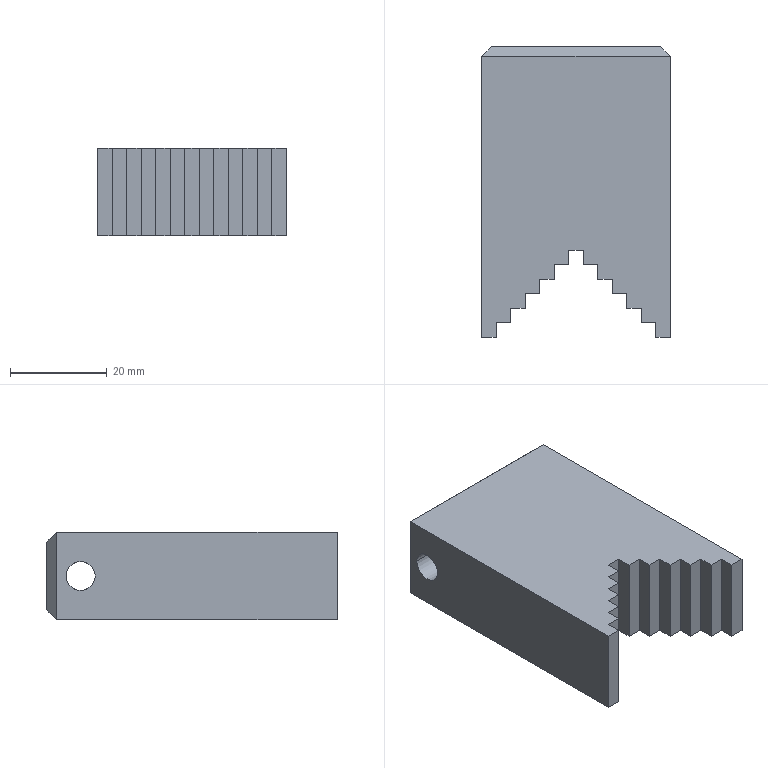Part | SolidWorks | features Chamfer 1, Extrusion 1, ICE 1, RevCut 1 | 1 solid | 42 faces | box 39 x 60 x 18 mm | volume 32904 mm3 | plane 34 | cylinder 6 | cone 2 | commonest cylinder face diameters 6 x4 12 x2
STEP:
#1=CARTESIAN_POINT('',(0.,0.2573,0.));
#2=VERTEX_POINT('',#1);
#3=CARTESIAN_POINT('',(0.,0.3937,0.2362));
#4=VERTEX_POINT('',#3);
#5=CARTESIAN_POINT('',(0.,0.2573,0.));
#6=DIRECTION('',(0.,0.5,0.866));
#7=VECTOR('',#6,39.37);
#8=LINE('',#5,#7);
#9=EDGE_CURVE('',#2,#4,#8,.T.);
#10=ORIENTED_EDGE('',*,*,#9,.F.);
#11=CARTESIAN_POINT('',(0.,0.3937,-0.2362));
#12=VERTEX_POINT('',#11);
#13=CARTESIAN_POINT('',(0.,0.2573,0.));
#14=DIRECTION('',(0.,0.5,-0.866));
#15=VECTOR('',#14,39.37);
#16=LINE('',#13,#15);
#17=EDGE_CURVE('',#2,#12,#16,.T.);
#18=ORIENTED_EDGE('',*,*,#17,.T.);
#19=CARTESIAN_POINT('',(0.,0.3937,0.));
#20=DIRECTION('',(0.,1.,0.));
#21=DIRECTION('',(0.,0.,1.));
#22=AXIS2_PLACEMENT_3D('',#19,#20,#21);
#23=CIRCLE('',#22,0.2362);
#24=EDGE_CURVE('',#12,#4,#23,.T.);
#25=ORIENTED_EDGE('',*,*,#24,.T.);
#26=EDGE_LOOP('',(#10,#18,#25));
#27=FACE_OUTER_BOUND('',#26,.T.);
#28=CARTESIAN_POINT('',(0.,39.627,0.));
#29=DIRECTION('',(0.,1.,0.));
#30=DIRECTION('',(0.,0.,1.));
#31=AXIS2_PLACEMENT_3D('',#28,#29,#30);
#32=CONICAL_SURFACE('',#31,68.191,1.047);
#33=ADVANCED_FACE('',(#27),#32,.F.);
#34=CARTESIAN_POINT('',(-0.2362,1.024,0.));
#35=VERTEX_POINT('',#34);
#36=CARTESIAN_POINT('',(-0.2362,0.7874,0.));
#37=VERTEX_POINT('',#36);
#38=CARTESIAN_POINT('',(-0.2362,1.024,0.));
#39=CARTESIAN_POINT('',(-0.2362,1.024,-0.007949));
#40=CARTESIAN_POINT('',(-0.2358,1.023,-0.01574));
#41=CARTESIAN_POINT('',(-0.2343,1.02,-0.03103));
#42=CARTESIAN_POINT('',(-0.2332,1.017,-0.0386));
#43=CARTESIAN_POINT('',(-0.2303,1.011,-0.05287));
#44=CARTESIAN_POINT('',(-0.2287,1.008,-0.05961));
#45=CARTESIAN_POINT('',(-0.225,0.9992,-0.07235));
#46=CARTESIAN_POINT('',(-0.223,0.9943,-0.07826));
#47=CARTESIAN_POINT('',(-0.2189,0.9836,-0.08896));
#48=CARTESIAN_POINT('',(-0.2168,0.9777,-0.09383));
#49=CARTESIAN_POINT('',(-0.2129,0.9649,-0.1024));
#50=CARTESIAN_POINT('',(-0.2111,0.9582,-0.106));
#51=CARTESIAN_POINT('',(-0.2081,0.9441,-0.1119));
#52=CARTESIAN_POINT('',(-0.2068,0.9365,-0.1142));
#53=CARTESIAN_POINT('',(-0.205,0.9212,-0.1173));
#54=CARTESIAN_POINT('',(-0.2046,0.9135,-0.1181));
#55=CARTESIAN_POINT('',(-0.2046,0.8978,-0.1181));
#56=CARTESIAN_POINT('',(-0.205,0.8898,-0.1173));
#57=CARTESIAN_POINT('',(-0.2068,0.8745,-0.1142));
#58=CARTESIAN_POINT('',(-0.208,0.867,-0.1119));
#59=CARTESIAN_POINT('',(-0.2112,0.8527,-0.1059));
#60=CARTESIAN_POINT('',(-0.213,0.846,-0.1023));
#61=CARTESIAN_POINT('',(-0.2169,0.8333,-0.09378));
#62=CARTESIAN_POINT('',(-0.2189,0.8274,-0.08888));
#63=CARTESIAN_POINT('',(-0.223,0.8166,-0.07817));
#64=CARTESIAN_POINT('',(-0.225,0.8118,-0.07231));
#65=CARTESIAN_POINT('',(-0.2287,0.8032,-0.05952));
#66=CARTESIAN_POINT('',(-0.2304,0.7996,-0.05274));
#67=CARTESIAN_POINT('',(-0.2332,0.7936,-0.03856));
#68=CARTESIAN_POINT('',(-0.2343,0.7913,-0.03106));
#69=CARTESIAN_POINT('',(-0.2358,0.7882,-0.01562));
#70=CARTESIAN_POINT('',(-0.2362,0.7874,-0.007842));
#71=CARTESIAN_POINT('',(-0.2362,0.7874,0.));
#72=B_SPLINE_CURVE_WITH_KNOTS('',3,(#38,#39,#40,#41,#42,#43,#44,#45,#46,#47,#48,#49,#50,#51,#52,#53,#54,#55,#56,#57,#58,#59,#60,#61,#62,#63,#64,#65,#66,#67,#68,#69,#70,#71),.UNSPECIFIED.,.F.,.F.,(4,2,2,2,2,2,2,2,2,2,2,2,2,2,2,2,4),(0.,0.0005964,0.001193,0.001789,0.002386,0.002982,0.003579,0.004175,0.004771,0.005368,0.005964,0.006561,0.007157,0.007754,0.00835,0.008947,0.009543),.UNSPECIFIED.);
#73=EDGE_CURVE('',#35,#37,#72,.T.);
#74=ORIENTED_EDGE('',*,*,#73,.T.);
#75=CARTESIAN_POINT('',(-0.2362,0.7874,0.));
#76=CARTESIAN_POINT('',(-0.2362,0.7874,0.007829));
#77=CARTESIAN_POINT('',(-0.2358,0.7882,0.0158));
#78=CARTESIAN_POINT('',(-0.2343,0.7913,0.0311));
#79=CARTESIAN_POINT('',(-0.2332,0.7936,0.03852));
#80=CARTESIAN_POINT('',(-0.2303,0.7996,0.05291));
#81=CARTESIAN_POINT('',(-0.2287,0.8033,0.05967));
#82=CARTESIAN_POINT('',(-0.225,0.8118,0.07232));
#83=CARTESIAN_POINT('',(-0.2229,0.8167,0.07827));
#84=CARTESIAN_POINT('',(-0.2189,0.8275,0.08899));
#85=CARTESIAN_POINT('',(-0.2169,0.8333,0.09379));
#86=CARTESIAN_POINT('',(-0.213,0.846,0.1023));
#87=CARTESIAN_POINT('',(-0.2111,0.8528,0.106));
#88=CARTESIAN_POINT('',(-0.2081,0.8669,0.1119));
#89=CARTESIAN_POINT('',(-0.2068,0.8743,0.1142));
#90=CARTESIAN_POINT('',(-0.205,0.8897,0.1173));
#91=CARTESIAN_POINT('',(-0.2046,0.8976,0.1181));
#92=CARTESIAN_POINT('',(-0.2046,0.9132,0.1181));
#93=CARTESIAN_POINT('',(-0.205,0.9211,0.1173));
#94=CARTESIAN_POINT('',(-0.2068,0.9365,0.1142));
#95=CARTESIAN_POINT('',(-0.208,0.9439,0.112));
#96=CARTESIAN_POINT('',(-0.2127,0.9653,0.103));
#97=CARTESIAN_POINT('',(-0.2169,0.9782,0.09436));
#98=CARTESIAN_POINT('',(-0.223,0.9943,0.07821));
#99=CARTESIAN_POINT('',(-0.225,0.9992,0.07237));
#100=CARTESIAN_POINT('',(-0.2286,1.008,0.05973));
#101=CARTESIAN_POINT('',(-0.2303,1.011,0.05285));
#102=CARTESIAN_POINT('',(-0.2332,1.017,0.03862));
#103=CARTESIAN_POINT('',(-0.2343,1.02,0.03124));
#104=CARTESIAN_POINT('',(-0.2358,1.023,0.01591));
#105=CARTESIAN_POINT('',(-0.2362,1.024,0.007935));
#106=CARTESIAN_POINT('',(-0.2362,1.024,0.));
#107=B_SPLINE_CURVE_WITH_KNOTS('',3,(#75,#76,#77,#78,#79,#80,#81,#82,#83,#84,#85,#86,#87,#88,#89,#90,#91,#92,#93,#94,#95,#96,#97,#98,#99,#100,#101,#102,#103,#104,#105,#106),.UNSPECIFIED.,.F.,.F.,(4,2,2,2,2,2,2,2,2,2,2,2,2,2,2,4),(0.009543,0.01014,0.01073,0.01133,0.01192,0.01252,0.01312,0.01371,0.01431,0.0149,0.0155,0.01669,0.01728,0.01788,0.01847,0.01907),.UNSPECIFIED.);
#108=EDGE_CURVE('',#37,#35,#107,.T.);
#109=ORIENTED_EDGE('',*,*,#108,.T.);
#110=EDGE_LOOP('',(#74,#109));
#111=FACE_BOUND('',#110,.T.);
#112=ORIENTED_EDGE('',*,*,#24,.F.);
#113=CARTESIAN_POINT('',(0.,1.181,-0.2362));
#114=VERTEX_POINT('',#113);
#115=CARTESIAN_POINT('',(0.,1.249,-0.2362));
#116=DIRECTION('',(0.,1.,0.));
#117=VECTOR('',#116,39.37);
#118=LINE('',#115,#117);
#119=EDGE_CURVE('',#12,#114,#118,.T.);
#120=ORIENTED_EDGE('',*,*,#119,.T.);
#121=CARTESIAN_POINT('',(0.,1.181,0.2362));
#122=VERTEX_POINT('',#121);
#123=CARTESIAN_POINT('',(0.,1.181,0.));
#124=DIRECTION('',(0.,1.,0.));
#125=DIRECTION('',(0.,0.,1.));
#126=AXIS2_PLACEMENT_3D('',#123,#124,#125);
#127=CIRCLE('',#126,0.2362);
#128=EDGE_CURVE('',#114,#122,#127,.T.);
#129=ORIENTED_EDGE('',*,*,#128,.T.);
#130=CARTESIAN_POINT('',(0.,1.249,0.2362));
#131=DIRECTION('',(0.,1.,0.));
#132=VECTOR('',#131,39.37);
#133=LINE('',#130,#132);
#134=EDGE_CURVE('',#4,#122,#133,.T.);
#135=ORIENTED_EDGE('',*,*,#134,.F.);
#136=EDGE_LOOP('',(#112,#120,#129,#135));
#137=FACE_OUTER_BOUND('',#136,.T.);
#138=CARTESIAN_POINT('',(0.,1.249,0.));
#139=DIRECTION('',(0.,1.,0.));
#140=DIRECTION('',(0.,0.,1.));
#141=AXIS2_PLACEMENT_3D('',#138,#139,#140);
#142=CYLINDRICAL_SURFACE('',#141,0.2362);
#143=ADVANCED_FACE('',(#111,#137),#142,.F.);
#144=CARTESIAN_POINT('',(0.2362,0.7874,0.));
#145=VERTEX_POINT('',#144);
#146=CARTESIAN_POINT('',(0.2362,1.024,0.));
#147=VERTEX_POINT('',#146);
#148=CARTESIAN_POINT('',(0.2362,0.7874,0.));
#149=CARTESIAN_POINT('',(0.2362,0.7874,-0.007829));
#150=CARTESIAN_POINT('',(0.2358,0.7882,-0.0158));
#151=CARTESIAN_POINT('',(0.2343,0.7913,-0.0311));
#152=CARTESIAN_POINT('',(0.2332,0.7936,-0.03852));
#153=CARTESIAN_POINT('',(0.2303,0.7996,-0.05291));
#154=CARTESIAN_POINT('',(0.2287,0.8033,-0.05967));
#155=CARTESIAN_POINT('',(0.225,0.8118,-0.07232));
#156=CARTESIAN_POINT('',(0.2229,0.8167,-0.07827));
#157=CARTESIAN_POINT('',(0.2189,0.8275,-0.08899));
#158=CARTESIAN_POINT('',(0.2169,0.8333,-0.09379));
#159=CARTESIAN_POINT('',(0.213,0.846,-0.1023));
#160=CARTESIAN_POINT('',(0.2111,0.8528,-0.106));
#161=CARTESIAN_POINT('',(0.2081,0.8669,-0.1119));
#162=CARTESIAN_POINT('',(0.2068,0.8743,-0.1142));
#163=CARTESIAN_POINT('',(0.205,0.8897,-0.1173));
#164=CARTESIAN_POINT('',(0.2046,0.8976,-0.1181));
#165=CARTESIAN_POINT('',(0.2046,0.9132,-0.1181));
#166=CARTESIAN_POINT('',(0.205,0.9211,-0.1173));
#167=CARTESIAN_POINT('',(0.2068,0.9365,-0.1142));
#168=CARTESIAN_POINT('',(0.208,0.9439,-0.112));
#169=CARTESIAN_POINT('',(0.2127,0.9653,-0.103));
#170=CARTESIAN_POINT('',(0.2169,0.9782,-0.09436));
#171=CARTESIAN_POINT('',(0.223,0.9943,-0.07821));
#172=CARTESIAN_POINT('',(0.225,0.9992,-0.07237));
#173=CARTESIAN_POINT('',(0.2286,1.008,-0.05973));
#174=CARTESIAN_POINT('',(0.2303,1.011,-0.05285));
#175=CARTESIAN_POINT('',(0.2332,1.017,-0.03862));
#176=CARTESIAN_POINT('',(0.2343,1.02,-0.03124));
#177=CARTESIAN_POINT('',(0.2358,1.023,-0.01591));
#178=CARTESIAN_POINT('',(0.2362,1.024,-0.007935));
#179=CARTESIAN_POINT('',(0.2362,1.024,0.));
#180=B_SPLINE_CURVE_WITH_KNOTS('',3,(#148,#149,#150,#151,#152,#153,#154,#155,#156,#157,#158,#159,#160,#161,#162,#163,#164,#165,#166,#167,#168,#169,#170,#171,#172,#173,#174,#175,#176,#177,#178,#179),.UNSPECIFIED.,.F.,.F.,(4,2,2,2,2,2,2,2,2,2,2,2,2,2,2,4),(0.009543,0.01014,0.01073,0.01133,0.01192,0.01252,0.01312,0.01371,0.01431,0.0149,0.0155,0.01669,0.01728,0.01788,0.01847,0.01907),.UNSPECIFIED.);
#181=EDGE_CURVE('',#145,#147,#180,.T.);
#182=ORIENTED_EDGE('',*,*,#181,.F.);
#183=CARTESIAN_POINT('',(0.7677,0.7874,0.));
#184=VERTEX_POINT('',#183);
#185=CARTESIAN_POINT('',(-0.7677,0.7874,0.));
#186=DIRECTION('',(1.,0.,0.));
#187=VECTOR('',#186,39.37);
#188=LINE('',#185,#187);
#189=EDGE_CURVE('',#145,#184,#188,.T.);
#190=ORIENTED_EDGE('',*,*,#189,.T.);
#191=CARTESIAN_POINT('',(0.7677,1.024,0.));
#192=VERTEX_POINT('',#191);
#193=CARTESIAN_POINT('',(0.7677,0.9055,0.));
#194=DIRECTION('',(1.,0.,0.));
#195=DIRECTION('',(0.,1.,0.));
#196=AXIS2_PLACEMENT_3D('',#193,#194,#195);
#197=CIRCLE('',#196,0.1181);
#198=EDGE_CURVE('',#184,#192,#197,.T.);
#199=ORIENTED_EDGE('',*,*,#198,.T.);
#200=CARTESIAN_POINT('',(-0.7677,1.024,0.));
#201=DIRECTION('',(1.,0.,0.));
#202=VECTOR('',#201,39.37);
#203=LINE('',#200,#202);
#204=EDGE_CURVE('',#147,#192,#203,.T.);
#205=ORIENTED_EDGE('',*,*,#204,.F.);
#206=EDGE_LOOP('',(#182,#190,#199,#205));
#207=FACE_OUTER_BOUND('',#206,.T.);
#208=CARTESIAN_POINT('',(-0.7677,0.9055,0.));
#209=DIRECTION('',(1.,0.,0.));
#210=DIRECTION('',(0.,1.,0.));
#211=AXIS2_PLACEMENT_3D('',#208,#209,#210);
#212=CYLINDRICAL_SURFACE('',#211,0.1181);
#213=ADVANCED_FACE('',(#207),#212,.F.);
#214=CARTESIAN_POINT('',(-0.7677,0.7874,0.));
#215=VERTEX_POINT('',#214);
#216=CARTESIAN_POINT('',(-0.7677,1.024,0.));
#217=VERTEX_POINT('',#216);
#218=CARTESIAN_POINT('',(-0.7677,0.9055,0.));
#219=DIRECTION('',(1.,0.,0.));
#220=DIRECTION('',(0.,1.,0.));
#221=AXIS2_PLACEMENT_3D('',#218,#219,#220);
#222=CIRCLE('',#221,0.1181);
#223=EDGE_CURVE('',#215,#217,#222,.T.);
#224=ORIENTED_EDGE('',*,*,#223,.F.);
#225=CARTESIAN_POINT('',(-0.7677,0.7874,0.));
#226=DIRECTION('',(1.,0.,0.));
#227=VECTOR('',#226,39.37);
#228=LINE('',#225,#227);
#229=EDGE_CURVE('',#215,#37,#228,.T.);
#230=ORIENTED_EDGE('',*,*,#229,.T.);
#231=ORIENTED_EDGE('',*,*,#73,.F.);
#232=CARTESIAN_POINT('',(-0.7677,1.024,0.));
#233=DIRECTION('',(1.,0.,0.));
#234=VECTOR('',#233,39.37);
#235=LINE('',#232,#234);
#236=EDGE_CURVE('',#217,#35,#235,.T.);
#237=ORIENTED_EDGE('',*,*,#236,.F.);
#238=EDGE_LOOP('',(#224,#230,#231,#237));
#239=FACE_OUTER_BOUND('',#238,.T.);
#240=CARTESIAN_POINT('',(-0.7677,0.9055,0.));
#241=DIRECTION('',(1.,0.,0.));
#242=DIRECTION('',(0.,1.,0.));
#243=AXIS2_PLACEMENT_3D('',#240,#241,#242);
#244=CYLINDRICAL_SURFACE('',#243,0.1181);
#245=ADVANCED_FACE('',(#239),#244,.F.);
#246=ORIENTED_EDGE('',*,*,#229,.F.);
#247=CARTESIAN_POINT('',(-0.7677,0.9055,0.));
#248=DIRECTION('',(1.,0.,0.));
#249=DIRECTION('',(0.,1.,0.));
#250=AXIS2_PLACEMENT_3D('',#247,#248,#249);
#251=CIRCLE('',#250,0.1181);
#252=EDGE_CURVE('',#217,#215,#251,.T.);
#253=ORIENTED_EDGE('',*,*,#252,.F.);
#254=ORIENTED_EDGE('',*,*,#236,.T.);
#255=ORIENTED_EDGE('',*,*,#108,.F.);
#256=EDGE_LOOP('',(#246,#253,#254,#255));
#257=FACE_OUTER_BOUND('',#256,.T.);
#258=CARTESIAN_POINT('',(-0.7677,0.9055,0.));
#259=DIRECTION('',(1.,0.,0.));
#260=DIRECTION('',(0.,1.,0.));
#261=AXIS2_PLACEMENT_3D('',#258,#259,#260);
#262=CYLINDRICAL_SURFACE('',#261,0.1181);
#263=ADVANCED_FACE('',(#257),#262,.F.);
#264=ORIENTED_EDGE('',*,*,#189,.F.);
#265=CARTESIAN_POINT('',(0.2362,1.024,0.));
#266=CARTESIAN_POINT('',(0.2362,1.024,0.007949));
#267=CARTESIAN_POINT('',(0.2358,1.023,0.01574));
#268=CARTESIAN_POINT('',(0.2343,1.02,0.03103));
#269=CARTESIAN_POINT('',(0.2332,1.017,0.0386));
#270=CARTESIAN_POINT('',(0.2303,1.011,0.05287));
#271=CARTESIAN_POINT('',(0.2287,1.008,0.05961));
#272=CARTESIAN_POINT('',(0.225,0.9992,0.07235));
#273=CARTESIAN_POINT('',(0.223,0.9943,0.07826));
#274=CARTESIAN_POINT('',(0.2189,0.9836,0.08896));
#275=CARTESIAN_POINT('',(0.2168,0.9777,0.09383));
#276=CARTESIAN_POINT('',(0.2129,0.9649,0.1024));
#277=CARTESIAN_POINT('',(0.2111,0.9582,0.106));
#278=CARTESIAN_POINT('',(0.2081,0.9441,0.1119));
#279=CARTESIAN_POINT('',(0.2068,0.9365,0.1142));
#280=CARTESIAN_POINT('',(0.205,0.9212,0.1173));
#281=CARTESIAN_POINT('',(0.2046,0.9135,0.1181));
#282=CARTESIAN_POINT('',(0.2046,0.8978,0.1181));
#283=CARTESIAN_POINT('',(0.205,0.8898,0.1173));
#284=CARTESIAN_POINT('',(0.2068,0.8745,0.1142));
#285=CARTESIAN_POINT('',(0.208,0.867,0.1119));
#286=CARTESIAN_POINT('',(0.2112,0.8527,0.1059));
#287=CARTESIAN_POINT('',(0.213,0.846,0.1023));
#288=CARTESIAN_POINT('',(0.2169,0.8333,0.09378));
#289=CARTESIAN_POINT('',(0.2189,0.8274,0.08888));
#290=CARTESIAN_POINT('',(0.223,0.8166,0.07817));
#291=CARTESIAN_POINT('',(0.225,0.8118,0.07231));
#292=CARTESIAN_POINT('',(0.2287,0.8032,0.05952));
#293=CARTESIAN_POINT('',(0.2304,0.7996,0.05274));
#294=CARTESIAN_POINT('',(0.2332,0.7936,0.03856));
#295=CARTESIAN_POINT('',(0.2343,0.7913,0.03106));
#296=CARTESIAN_POINT('',(0.2358,0.7882,0.01562));
#297=CARTESIAN_POINT('',(0.2362,0.7874,0.007842));
#298=CARTESIAN_POINT('',(0.2362,0.7874,0.));
#299=B_SPLINE_CURVE_WITH_KNOTS('',3,(#265,#266,#267,#268,#269,#270,#271,#272,#273,#274,#275,#276,#277,#278,#279,#280,#281,#282,#283,#284,#285,#286,#287,#288,#289,#290,#291,#292,#293,#294,#295,#296,#297,#298),.UNSPECIFIED.,.F.,.F.,(4,2,2,2,2,2,2,2,2,2,2,2,2,2,2,2,4),(0.,0.0005964,0.001193,0.001789,0.002386,0.002982,0.003579,0.004175,0.004771,0.005368,0.005964,0.006561,0.007157,0.007754,0.00835,0.008947,0.009543),.UNSPECIFIED.);
#300=EDGE_CURVE('',#147,#145,#299,.T.);
#301=ORIENTED_EDGE('',*,*,#300,.F.);
#302=ORIENTED_EDGE('',*,*,#204,.T.);
#303=CARTESIAN_POINT('',(0.7677,0.9055,0.));
#304=DIRECTION('',(1.,0.,0.));
#305=DIRECTION('',(0.,1.,0.));
#306=AXIS2_PLACEMENT_3D('',#303,#304,#305);
#307=CIRCLE('',#306,0.1181);
#308=EDGE_CURVE('',#192,#184,#307,.T.);
#309=ORIENTED_EDGE('',*,*,#308,.T.);
#310=EDGE_LOOP('',(#264,#301,#302,#309));
#311=FACE_OUTER_BOUND('',#310,.T.);
#312=CARTESIAN_POINT('',(-0.7677,0.9055,0.));
#313=DIRECTION('',(1.,0.,0.));
#314=DIRECTION('',(0.,1.,0.));
#315=AXIS2_PLACEMENT_3D('',#312,#313,#314);
#316=CYLINDRICAL_SURFACE('',#315,0.1181);
#317=ADVANCED_FACE('',(#311),#316,.F.);
#318=CARTESIAN_POINT('',(0.6496,-1.181,-0.3543));
#319=VERTEX_POINT('',#318);
#320=CARTESIAN_POINT('',(0.7677,-1.181,-0.3543));
#321=VERTEX_POINT('',#320);
#322=CARTESIAN_POINT('',(0.6496,-1.181,-0.3543));
#323=DIRECTION('',(1.,0.,0.));
#324=VECTOR('',#323,39.37);
#325=LINE('',#322,#324);
#326=EDGE_CURVE('',#319,#321,#325,.T.);
#327=ORIENTED_EDGE('',*,*,#326,.T.);
#328=CARTESIAN_POINT('',(0.7677,-1.181,0.3543));
#329=VERTEX_POINT('',#328);
#330=CARTESIAN_POINT('',(0.7677,-1.181,0.3543));
#331=DIRECTION('',(0.,0.,-1.));
#332=VECTOR('',#331,39.37);
#333=LINE('',#330,#332);
#334=EDGE_CURVE('',#329,#321,#333,.T.);
#335=ORIENTED_EDGE('',*,*,#334,.F.);
#336=CARTESIAN_POINT('',(0.6496,-1.181,0.3543));
#337=VERTEX_POINT('',#336);
#338=CARTESIAN_POINT('',(0.6496,-1.181,0.3543));
#339=DIRECTION('',(1.,0.,0.));
#340=VECTOR('',#339,39.37);
#341=LINE('',#338,#340);
#342=EDGE_CURVE('',#337,#329,#341,.T.);
#343=ORIENTED_EDGE('',*,*,#342,.F.);
#344=CARTESIAN_POINT('',(0.6496,-1.181,0.3543));
#345=DIRECTION('',(0.,0.,-1.));
#346=VECTOR('',#345,39.37);
#347=LINE('',#344,#346);
#348=EDGE_CURVE('',#337,#319,#347,.T.);
#349=ORIENTED_EDGE('',*,*,#348,.T.);
#350=EDGE_LOOP('',(#327,#335,#343,#349));
#351=FACE_OUTER_BOUND('',#350,.T.);
#352=CARTESIAN_POINT('',(0.6496,-1.181,0.3543));
#353=DIRECTION('',(0.,1.,0.));
#354=DIRECTION('',(0.,0.,1.));
#355=AXIS2_PLACEMENT_3D('',#352,#353,#354);
#356=PLANE('',#355);
#357=ADVANCED_FACE('',(#351),#356,.F.);
#358=ORIENTED_EDGE('',*,*,#308,.F.);
#359=ORIENTED_EDGE('',*,*,#198,.F.);
#360=EDGE_LOOP('',(#358,#359));
#361=FACE_BOUND('',#360,.T.);
#362=CARTESIAN_POINT('',(0.7677,1.102,-0.3543));
#363=VERTEX_POINT('',#362);
#364=CARTESIAN_POINT('',(0.7677,1.181,-0.3543));
#365=DIRECTION('',(0.,1.,0.));
#366=VECTOR('',#365,39.37);
#367=LINE('',#364,#366);
#368=EDGE_CURVE('',#321,#363,#367,.T.);
#369=ORIENTED_EDGE('',*,*,#368,.T.);
#370=CARTESIAN_POINT('',(0.7677,1.102,0.3543));
#371=VERTEX_POINT('',#370);
#372=CARTESIAN_POINT('',(0.7677,1.102,0.3543));
#373=DIRECTION('',(0.,0.,1.));
#374=VECTOR('',#373,39.37);
#375=LINE('',#372,#374);
#376=EDGE_CURVE('',#363,#371,#375,.T.);
#377=ORIENTED_EDGE('',*,*,#376,.T.);
#378=CARTESIAN_POINT('',(0.7677,1.181,0.3543));
#379=DIRECTION('',(0.,1.,0.));
#380=VECTOR('',#379,39.37);
#381=LINE('',#378,#380);
#382=EDGE_CURVE('',#329,#371,#381,.T.);
#383=ORIENTED_EDGE('',*,*,#382,.F.);
#384=ORIENTED_EDGE('',*,*,#334,.T.);
#385=EDGE_LOOP('',(#369,#377,#383,#384));
#386=FACE_OUTER_BOUND('',#385,.T.);
#387=CARTESIAN_POINT('',(0.7677,1.181,0.3543));
#388=DIRECTION('',(-1.,0.,0.));
#389=DIRECTION('',(0.,-1.,0.));
#390=AXIS2_PLACEMENT_3D('',#387,#388,#389);
#391=PLANE('',#390);
#392=ADVANCED_FACE('',(#361,#386),#391,.F.);
#393=CARTESIAN_POINT('',(0.,1.181,0.));
#394=DIRECTION('',(0.,1.,0.));
#395=DIRECTION('',(0.,0.,1.));
#396=AXIS2_PLACEMENT_3D('',#393,#394,#395);
#397=CIRCLE('',#396,0.2362);
#398=EDGE_CURVE('',#122,#114,#397,.T.);
#399=ORIENTED_EDGE('',*,*,#398,.F.);
#400=ORIENTED_EDGE('',*,*,#128,.F.);
#401=EDGE_LOOP('',(#399,#400));
#402=FACE_BOUND('',#401,.T.);
#403=CARTESIAN_POINT('',(-0.689,1.181,0.2756));
#404=VERTEX_POINT('',#403);
#405=CARTESIAN_POINT('',(0.689,1.181,0.2756));
#406=VERTEX_POINT('',#405);
#407=CARTESIAN_POINT('',(-0.7677,1.181,0.2756));
#408=DIRECTION('',(1.,0.,0.));
#409=VECTOR('',#408,39.37);
#410=LINE('',#407,#409);
#411=EDGE_CURVE('',#404,#406,#410,.T.);
#412=ORIENTED_EDGE('',*,*,#411,.T.);
#413=CARTESIAN_POINT('',(0.689,1.181,-0.2756));
#414=VERTEX_POINT('',#413);
#415=CARTESIAN_POINT('',(0.689,1.181,0.3543));
#416=DIRECTION('',(0.,0.,-1.));
#417=VECTOR('',#416,39.37);
#418=LINE('',#415,#417);
#419=EDGE_CURVE('',#406,#414,#418,.T.);
#420=ORIENTED_EDGE('',*,*,#419,.T.);
#421=CARTESIAN_POINT('',(-0.689,1.181,-0.2756));
#422=VERTEX_POINT('',#421);
#423=CARTESIAN_POINT('',(-0.7677,1.181,-0.2756));
#424=DIRECTION('',(-1.,0.,0.));
#425=VECTOR('',#424,39.37);
#426=LINE('',#423,#425);
#427=EDGE_CURVE('',#414,#422,#426,.T.);
#428=ORIENTED_EDGE('',*,*,#427,.T.);
#429=CARTESIAN_POINT('',(-0.689,1.181,0.3543));
#430=DIRECTION('',(0.,0.,1.));
#431=VECTOR('',#430,39.37);
#432=LINE('',#429,#431);
#433=EDGE_CURVE('',#422,#404,#432,.T.);
#434=ORIENTED_EDGE('',*,*,#433,.T.);
#435=EDGE_LOOP('',(#412,#420,#428,#434));
#436=FACE_OUTER_BOUND('',#435,.T.);
#437=CARTESIAN_POINT('',(-0.7677,1.181,0.3543));
#438=DIRECTION('',(0.,-1.,0.));
#439=DIRECTION('',(0.,0.,-1.));
#440=AXIS2_PLACEMENT_3D('',#437,#438,#439);
#441=PLANE('',#440);
#442=ADVANCED_FACE('',(#402,#436),#441,.F.);
#443=ORIENTED_EDGE('',*,*,#252,.T.);
#444=ORIENTED_EDGE('',*,*,#223,.T.);
#445=EDGE_LOOP('',(#443,#444));
#446=FACE_BOUND('',#445,.T.);
#447=CARTESIAN_POINT('',(-0.7677,1.102,0.3543));
#448=VERTEX_POINT('',#447);
#449=CARTESIAN_POINT('',(-0.7677,-1.181,0.3543));
#450=VERTEX_POINT('',#449);
#451=CARTESIAN_POINT('',(-0.7677,1.181,0.3543));
#452=DIRECTION('',(0.,-1.,0.));
#453=VECTOR('',#452,39.37);
#454=LINE('',#451,#453);
#455=EDGE_CURVE('',#448,#450,#454,.T.);
#456=ORIENTED_EDGE('',*,*,#455,.F.);
#457=CARTESIAN_POINT('',(-0.7677,1.102,-0.3543));
#458=VERTEX_POINT('',#457);
#459=CARTESIAN_POINT('',(-0.7677,1.102,0.3543));
#460=DIRECTION('',(0.,0.,-1.));
#461=VECTOR('',#460,39.37);
#462=LINE('',#459,#461);
#463=EDGE_CURVE('',#448,#458,#462,.T.);
#464=ORIENTED_EDGE('',*,*,#463,.T.);
#465=CARTESIAN_POINT('',(-0.7677,-1.181,-0.3543));
#466=VERTEX_POINT('',#465);
#467=CARTESIAN_POINT('',(-0.7677,1.181,-0.3543));
#468=DIRECTION('',(0.,-1.,0.));
#469=VECTOR('',#468,39.37);
#470=LINE('',#467,#469);
#471=EDGE_CURVE('',#458,#466,#470,.T.);
#472=ORIENTED_EDGE('',*,*,#471,.T.);
#473=CARTESIAN_POINT('',(-0.7677,-1.181,0.3543));
#474=DIRECTION('',(0.,0.,-1.));
#475=VECTOR('',#474,39.37);
#476=LINE('',#473,#475);
#477=EDGE_CURVE('',#450,#466,#476,.T.);
#478=ORIENTED_EDGE('',*,*,#477,.F.);
#479=EDGE_LOOP('',(#456,#464,#472,#478));
#480=FACE_OUTER_BOUND('',#479,.T.);
#481=CARTESIAN_POINT('',(-0.7677,1.181,0.3543));
#482=DIRECTION('',(1.,0.,0.));
#483=DIRECTION('',(0.,1.,0.));
#484=AXIS2_PLACEMENT_3D('',#481,#482,#483);
#485=PLANE('',#484);
#486=ADVANCED_FACE('',(#446,#480),#485,.F.);
#487=CARTESIAN_POINT('',(-0.6496,-1.181,-0.3543));
#488=VERTEX_POINT('',#487);
#489=CARTESIAN_POINT('',(-0.7677,-1.181,-0.3543));
#490=DIRECTION('',(1.,0.,0.));
#491=VECTOR('',#490,39.37);
#492=LINE('',#489,#491);
#493=EDGE_CURVE('',#466,#488,#492,.T.);
#494=ORIENTED_EDGE('',*,*,#493,.T.);
#495=CARTESIAN_POINT('',(-0.6496,-1.181,0.3543));
#496=VERTEX_POINT('',#495);
#497=CARTESIAN_POINT('',(-0.6496,-1.181,0.3543));
#498=DIRECTION('',(0.,0.,-1.));
#499=VECTOR('',#498,39.37);
#500=LINE('',#497,#499);
#501=EDGE_CURVE('',#496,#488,#500,.T.);
#502=ORIENTED_EDGE('',*,*,#501,.F.);
#503=CARTESIAN_POINT('',(-0.7677,-1.181,0.3543));
#504=DIRECTION('',(1.,0.,0.));
#505=VECTOR('',#504,39.37);
#506=LINE('',#503,#505);
#507=EDGE_CURVE('',#450,#496,#506,.T.);
#508=ORIENTED_EDGE('',*,*,#507,.F.);
#509=ORIENTED_EDGE('',*,*,#477,.T.);
#510=EDGE_LOOP('',(#494,#502,#508,#509));
#511=FACE_OUTER_BOUND('',#510,.T.);
#512=CARTESIAN_POINT('',(-0.7677,-1.181,0.3543));
#513=DIRECTION('',(0.,1.,0.));
#514=DIRECTION('',(0.,0.,1.));
#515=AXIS2_PLACEMENT_3D('',#512,#513,#514);
#516=PLANE('',#515);
#517=ADVANCED_FACE('',(#511),#516,.F.);
#518=CARTESIAN_POINT('',(-0.6496,-1.063,-0.3543));
#519=VERTEX_POINT('',#518);
#520=CARTESIAN_POINT('',(-0.6496,-1.181,-0.3543));
#521=DIRECTION('',(0.,1.,0.));
#522=VECTOR('',#521,39.37);
#523=LINE('',#520,#522);
#524=EDGE_CURVE('',#488,#519,#523,.T.);
#525=ORIENTED_EDGE('',*,*,#524,.T.);
#526=CARTESIAN_POINT('',(-0.6496,-1.063,0.3543));
#527=VERTEX_POINT('',#526);
#528=CARTESIAN_POINT('',(-0.6496,-1.063,0.3543));
#529=DIRECTION('',(0.,0.,-1.));
#530=VECTOR('',#529,39.37);
#531=LINE('',#528,#530);
#532=EDGE_CURVE('',#527,#519,#531,.T.);
#533=ORIENTED_EDGE('',*,*,#532,.F.);
#534=CARTESIAN_POINT('',(-0.6496,-1.181,0.3543));
#535=DIRECTION('',(0.,1.,0.));
#536=VECTOR('',#535,39.37);
#537=LINE('',#534,#536);
#538=EDGE_CURVE('',#496,#527,#537,.T.);
#539=ORIENTED_EDGE('',*,*,#538,.F.);
#540=ORIENTED_EDGE('',*,*,#501,.T.);
#541=EDGE_LOOP('',(#525,#533,#539,#540));
#542=FACE_OUTER_BOUND('',#541,.T.);
#543=CARTESIAN_POINT('',(-0.6496,-1.181,0.3543));
#544=DIRECTION('',(-1.,0.,0.));
#545=DIRECTION('',(0.,0.,1.));
#546=AXIS2_PLACEMENT_3D('',#543,#544,#545);
#547=PLANE('',#546);
#548=ADVANCED_FACE('',(#542),#547,.F.);
#549=CARTESIAN_POINT('',(-0.5315,-1.063,-0.3543));
#550=VERTEX_POINT('',#549);
#551=CARTESIAN_POINT('',(-0.6496,-1.063,-0.3543));
#552=DIRECTION('',(1.,0.,0.));
#553=VECTOR('',#552,39.37);
#554=LINE('',#551,#553);
#555=EDGE_CURVE('',#519,#550,#554,.T.);
#556=ORIENTED_EDGE('',*,*,#555,.T.);
#557=CARTESIAN_POINT('',(-0.5315,-1.063,0.3543));
#558=VERTEX_POINT('',#557);
#559=CARTESIAN_POINT('',(-0.5315,-1.063,0.3543));
#560=DIRECTION('',(0.,0.,-1.));
#561=VECTOR('',#560,39.37);
#562=LINE('',#559,#561);
#563=EDGE_CURVE('',#558,#550,#562,.T.);
#564=ORIENTED_EDGE('',*,*,#563,.F.);
#565=CARTESIAN_POINT('',(-0.6496,-1.063,0.3543));
#566=DIRECTION('',(1.,0.,0.));
#567=VECTOR('',#566,39.37);
#568=LINE('',#565,#567);
#569=EDGE_CURVE('',#527,#558,#568,.T.);
#570=ORIENTED_EDGE('',*,*,#569,.F.);
#571=ORIENTED_EDGE('',*,*,#532,.T.);
#572=EDGE_LOOP('',(#556,#564,#570,#571));
#573=FACE_OUTER_BOUND('',#572,.T.);
#574=CARTESIAN_POINT('',(-0.6496,-1.063,0.3543));
#575=DIRECTION('',(0.,1.,0.));
#576=DIRECTION('',(0.,0.,1.));
#577=AXIS2_PLACEMENT_3D('',#574,#575,#576);
#578=PLANE('',#577);
#579=ADVANCED_FACE('',(#573),#578,.F.);
#580=CARTESIAN_POINT('',(-0.5315,-0.9449,-0.3543));
#581=VERTEX_POINT('',#580);
#582=CARTESIAN_POINT('',(-0.5315,-1.063,-0.3543));
#583=DIRECTION('',(0.,1.,0.));
#584=VECTOR('',#583,39.37);
#585=LINE('',#582,#584);
#586=EDGE_CURVE('',#550,#581,#585,.T.);
#587=ORIENTED_EDGE('',*,*,#586,.T.);
#588=CARTESIAN_POINT('',(-0.5315,-0.9449,0.3543));
#589=VERTEX_POINT('',#588);
#590=CARTESIAN_POINT('',(-0.5315,-0.9449,0.3543));
#591=DIRECTION('',(0.,0.,-1.));
#592=VECTOR('',#591,39.37);
#593=LINE('',#590,#592);
#594=EDGE_CURVE('',#589,#581,#593,.T.);
#595=ORIENTED_EDGE('',*,*,#594,.F.);
#596=CARTESIAN_POINT('',(-0.5315,-1.063,0.3543));
#597=DIRECTION('',(0.,1.,0.));
#598=VECTOR('',#597,39.37);
#599=LINE('',#596,#598);
#600=EDGE_CURVE('',#558,#589,#599,.T.);
#601=ORIENTED_EDGE('',*,*,#600,.F.);
#602=ORIENTED_EDGE('',*,*,#563,.T.);
#603=EDGE_LOOP('',(#587,#595,#601,#602));
#604=FACE_OUTER_BOUND('',#603,.T.);
#605=CARTESIAN_POINT('',(-0.5315,-1.063,0.3543));
#606=DIRECTION('',(-1.,0.,0.));
#607=DIRECTION('',(0.,0.,1.));
#608=AXIS2_PLACEMENT_3D('',#605,#606,#607);
#609=PLANE('',#608);
#610=ADVANCED_FACE('',(#604),#609,.F.);
#611=CARTESIAN_POINT('',(-0.4134,-0.9449,-0.3543));
#612=VERTEX_POINT('',#611);
#613=CARTESIAN_POINT('',(-0.5315,-0.9449,-0.3543));
#614=DIRECTION('',(1.,0.,0.));
#615=VECTOR('',#614,39.37);
#616=LINE('',#613,#615);
#617=EDGE_CURVE('',#581,#612,#616,.T.);
#618=ORIENTED_EDGE('',*,*,#617,.T.);
#619=CARTESIAN_POINT('',(-0.4134,-0.9449,0.3543));
#620=VERTEX_POINT('',#619);
#621=CARTESIAN_POINT('',(-0.4134,-0.9449,0.3543));
#622=DIRECTION('',(0.,0.,-1.));
#623=VECTOR('',#622,39.37);
#624=LINE('',#621,#623);
#625=EDGE_CURVE('',#620,#612,#624,.T.);
#626=ORIENTED_EDGE('',*,*,#625,.F.);
#627=CARTESIAN_POINT('',(-0.5315,-0.9449,0.3543));
#628=DIRECTION('',(1.,0.,0.));
#629=VECTOR('',#628,39.37);
#630=LINE('',#627,#629);
#631=EDGE_CURVE('',#589,#620,#630,.T.);
#632=ORIENTED_EDGE('',*,*,#631,.F.);
#633=ORIENTED_EDGE('',*,*,#594,.T.);
#634=EDGE_LOOP('',(#618,#626,#632,#633));
#635=FACE_OUTER_BOUND('',#634,.T.);
#636=CARTESIAN_POINT('',(-0.5315,-0.9449,0.3543));
#637=DIRECTION('',(0.,1.,0.));
#638=DIRECTION('',(0.,0.,1.));
#639=AXIS2_PLACEMENT_3D('',#636,#637,#638);
#640=PLANE('',#639);
#641=ADVANCED_FACE('',(#635),#640,.F.);
#642=CARTESIAN_POINT('',(-0.4134,-0.8268,-0.3543));
#643=VERTEX_POINT('',#642);
#644=CARTESIAN_POINT('',(-0.4134,-0.9449,-0.3543));
#645=DIRECTION('',(0.,1.,0.));
#646=VECTOR('',#645,39.37);
#647=LINE('',#644,#646);
#648=EDGE_CURVE('',#612,#643,#647,.T.);
#649=ORIENTED_EDGE('',*,*,#648,.T.);
#650=CARTESIAN_POINT('',(-0.4134,-0.8268,0.3543));
#651=VERTEX_POINT('',#650);
#652=CARTESIAN_POINT('',(-0.4134,-0.8268,0.3543));
#653=DIRECTION('',(0.,0.,-1.));
#654=VECTOR('',#653,39.37);
#655=LINE('',#652,#654);
#656=EDGE_CURVE('',#651,#643,#655,.T.);
#657=ORIENTED_EDGE('',*,*,#656,.F.);
#658=CARTESIAN_POINT('',(-0.4134,-0.9449,0.3543));
#659=DIRECTION('',(0.,1.,0.));
#660=VECTOR('',#659,39.37);
#661=LINE('',#658,#660);
#662=EDGE_CURVE('',#620,#651,#661,.T.);
#663=ORIENTED_EDGE('',*,*,#662,.F.);
#664=ORIENTED_EDGE('',*,*,#625,.T.);
#665=EDGE_LOOP('',(#649,#657,#663,#664));
#666=FACE_OUTER_BOUND('',#665,.T.);
#667=CARTESIAN_POINT('',(-0.4134,-0.9449,0.3543));
#668=DIRECTION('',(-1.,0.,0.));
#669=DIRECTION('',(0.,0.,1.));
#670=AXIS2_PLACEMENT_3D('',#667,#668,#669);
#671=PLANE('',#670);
#672=ADVANCED_FACE('',(#666),#671,.F.);
#673=CARTESIAN_POINT('',(-0.2953,-0.8268,-0.3543));
#674=VERTEX_POINT('',#673);
#675=CARTESIAN_POINT('',(-0.4134,-0.8268,-0.3543));
#676=DIRECTION('',(1.,0.,0.));
#677=VECTOR('',#676,39.37);
#678=LINE('',#675,#677);
#679=EDGE_CURVE('',#643,#674,#678,.T.);
#680=ORIENTED_EDGE('',*,*,#679,.T.);
#681=CARTESIAN_POINT('',(-0.2953,-0.8268,0.3543));
#682=VERTEX_POINT('',#681);
#683=CARTESIAN_POINT('',(-0.2953,-0.8268,0.3543));
#684=DIRECTION('',(0.,0.,-1.));
#685=VECTOR('',#684,39.37);
#686=LINE('',#683,#685);
#687=EDGE_CURVE('',#682,#674,#686,.T.);
#688=ORIENTED_EDGE('',*,*,#687,.F.);
#689=CARTESIAN_POINT('',(-0.4134,-0.8268,0.3543));
#690=DIRECTION('',(1.,0.,0.));
#691=VECTOR('',#690,39.37);
#692=LINE('',#689,#691);
#693=EDGE_CURVE('',#651,#682,#692,.T.);
#694=ORIENTED_EDGE('',*,*,#693,.F.);
#695=ORIENTED_EDGE('',*,*,#656,.T.);
#696=EDGE_LOOP('',(#680,#688,#694,#695));
#697=FACE_OUTER_BOUND('',#696,.T.);
#698=CARTESIAN_POINT('',(-0.4134,-0.8268,0.3543));
#699=DIRECTION('',(0.,1.,0.));
#700=DIRECTION('',(0.,0.,1.));
#701=AXIS2_PLACEMENT_3D('',#698,#699,#700);
#702=PLANE('',#701);
#703=ADVANCED_FACE('',(#697),#702,.F.);
#704=CARTESIAN_POINT('',(-0.2953,-0.7087,-0.3543));
#705=VERTEX_POINT('',#704);
#706=CARTESIAN_POINT('',(-0.2953,-0.8268,-0.3543));
#707=DIRECTION('',(0.,1.,0.));
#708=VECTOR('',#707,39.37);
#709=LINE('',#706,#708);
#710=EDGE_CURVE('',#674,#705,#709,.T.);
#711=ORIENTED_EDGE('',*,*,#710,.T.);
#712=CARTESIAN_POINT('',(-0.2953,-0.7087,0.3543));
#713=VERTEX_POINT('',#712);
#714=CARTESIAN_POINT('',(-0.2953,-0.7087,0.3543));
#715=DIRECTION('',(0.,0.,-1.));
#716=VECTOR('',#715,39.37);
#717=LINE('',#714,#716);
#718=EDGE_CURVE('',#713,#705,#717,.T.);
#719=ORIENTED_EDGE('',*,*,#718,.F.);
#720=CARTESIAN_POINT('',(-0.2953,-0.8268,0.3543));
#721=DIRECTION('',(0.,1.,0.));
#722=VECTOR('',#721,39.37);
#723=LINE('',#720,#722);
#724=EDGE_CURVE('',#682,#713,#723,.T.);
#725=ORIENTED_EDGE('',*,*,#724,.F.);
#726=ORIENTED_EDGE('',*,*,#687,.T.);
#727=EDGE_LOOP('',(#711,#719,#725,#726));
#728=FACE_OUTER_BOUND('',#727,.T.);
#729=CARTESIAN_POINT('',(-0.2953,-0.8268,0.3543));
#730=DIRECTION('',(-1.,0.,0.));
#731=DIRECTION('',(0.,0.,1.));
#732=AXIS2_PLACEMENT_3D('',#729,#730,#731);
#733=PLANE('',#732);
#734=ADVANCED_FACE('',(#728),#733,.F.);
#735=CARTESIAN_POINT('',(-0.1772,-0.7087,-0.3543));
#736=VERTEX_POINT('',#735);
#737=CARTESIAN_POINT('',(-0.2953,-0.7087,-0.3543));
#738=DIRECTION('',(1.,0.,0.));
#739=VECTOR('',#738,39.37);
#740=LINE('',#737,#739);
#741=EDGE_CURVE('',#705,#736,#740,.T.);
#742=ORIENTED_EDGE('',*,*,#741,.T.);
#743=CARTESIAN_POINT('',(-0.1772,-0.7087,0.3543));
#744=VERTEX_POINT('',#743);
#745=CARTESIAN_POINT('',(-0.1772,-0.7087,0.3543));
#746=DIRECTION('',(0.,0.,-1.));
#747=VECTOR('',#746,39.37);
#748=LINE('',#745,#747);
#749=EDGE_CURVE('',#744,#736,#748,.T.);
#750=ORIENTED_EDGE('',*,*,#749,.F.);
#751=CARTESIAN_POINT('',(-0.2953,-0.7087,0.3543));
#752=DIRECTION('',(1.,0.,0.));
#753=VECTOR('',#752,39.37);
#754=LINE('',#751,#753);
#755=EDGE_CURVE('',#713,#744,#754,.T.);
#756=ORIENTED_EDGE('',*,*,#755,.F.);
#757=ORIENTED_EDGE('',*,*,#718,.T.);
#758=EDGE_LOOP('',(#742,#750,#756,#757));
#759=FACE_OUTER_BOUND('',#758,.T.);
#760=CARTESIAN_POINT('',(-0.2953,-0.7087,0.3543));
#761=DIRECTION('',(0.,1.,0.));
#762=DIRECTION('',(0.,0.,1.));
#763=AXIS2_PLACEMENT_3D('',#760,#761,#762);
#764=PLANE('',#763);
#765=ADVANCED_FACE('',(#759),#764,.F.);
#766=CARTESIAN_POINT('',(-0.1772,-0.5906,-0.3543));
#767=VERTEX_POINT('',#766);
#768=CARTESIAN_POINT('',(-0.1772,-0.7087,-0.3543));
#769=DIRECTION('',(0.,1.,0.));
#770=VECTOR('',#769,39.37);
#771=LINE('',#768,#770);
#772=EDGE_CURVE('',#736,#767,#771,.T.);
#773=ORIENTED_EDGE('',*,*,#772,.T.);
#774=CARTESIAN_POINT('',(-0.1772,-0.5906,0.3543));
#775=VERTEX_POINT('',#774);
#776=CARTESIAN_POINT('',(-0.1772,-0.5906,0.3543));
#777=DIRECTION('',(0.,0.,-1.));
#778=VECTOR('',#777,39.37);
#779=LINE('',#776,#778);
#780=EDGE_CURVE('',#775,#767,#779,.T.);
#781=ORIENTED_EDGE('',*,*,#780,.F.);
#782=CARTESIAN_POINT('',(-0.1772,-0.7087,0.3543));
#783=DIRECTION('',(0.,1.,0.));
#784=VECTOR('',#783,39.37);
#785=LINE('',#782,#784);
#786=EDGE_CURVE('',#744,#775,#785,.T.);
#787=ORIENTED_EDGE('',*,*,#786,.F.);
#788=ORIENTED_EDGE('',*,*,#749,.T.);
#789=EDGE_LOOP('',(#773,#781,#787,#788));
#790=FACE_OUTER_BOUND('',#789,.T.);
#791=CARTESIAN_POINT('',(-0.1772,-0.7087,0.3543));
#792=DIRECTION('',(-1.,0.,0.));
#793=DIRECTION('',(0.,0.,1.));
#794=AXIS2_PLACEMENT_3D('',#791,#792,#793);
#795=PLANE('',#794);
#796=ADVANCED_FACE('',(#790),#795,.F.);
#797=CARTESIAN_POINT('',(-0.05906,-0.5906,-0.3543));
#798=VERTEX_POINT('',#797);
#799=CARTESIAN_POINT('',(-0.1772,-0.5906,-0.3543));
#800=DIRECTION('',(1.,0.,0.));
#801=VECTOR('',#800,39.37);
#802=LINE('',#799,#801);
#803=EDGE_CURVE('',#767,#798,#802,.T.);
#804=ORIENTED_EDGE('',*,*,#803,.T.);
#805=CARTESIAN_POINT('',(-0.05906,-0.5906,0.3543));
#806=VERTEX_POINT('',#805);
#807=CARTESIAN_POINT('',(-0.05906,-0.5906,0.3543));
#808=DIRECTION('',(0.,0.,-1.));
#809=VECTOR('',#808,39.37);
#810=LINE('',#807,#809);
#811=EDGE_CURVE('',#806,#798,#810,.T.);
#812=ORIENTED_EDGE('',*,*,#811,.F.);
#813=CARTESIAN_POINT('',(-0.1772,-0.5906,0.3543));
#814=DIRECTION('',(1.,0.,0.));
#815=VECTOR('',#814,39.37);
#816=LINE('',#813,#815);
#817=EDGE_CURVE('',#775,#806,#816,.T.);
#818=ORIENTED_EDGE('',*,*,#817,.F.);
#819=ORIENTED_EDGE('',*,*,#780,.T.);
#820=EDGE_LOOP('',(#804,#812,#818,#819));
#821=FACE_OUTER_BOUND('',#820,.T.);
#822=CARTESIAN_POINT('',(-0.1772,-0.5906,0.3543));
#823=DIRECTION('',(0.,1.,0.));
#824=DIRECTION('',(0.,0.,1.));
#825=AXIS2_PLACEMENT_3D('',#822,#823,#824);
#826=PLANE('',#825);
#827=ADVANCED_FACE('',(#821),#826,.F.);
#828=CARTESIAN_POINT('',(-0.05906,-0.4724,-0.3543));
#829=VERTEX_POINT('',#828);
#830=CARTESIAN_POINT('',(-0.05906,-0.5906,-0.3543));
#831=DIRECTION('',(0.,1.,0.));
#832=VECTOR('',#831,39.37);
#833=LINE('',#830,#832);
#834=EDGE_CURVE('',#798,#829,#833,.T.);
#835=ORIENTED_EDGE('',*,*,#834,.T.);
#836=CARTESIAN_POINT('',(-0.05906,-0.4724,0.3543));
#837=VERTEX_POINT('',#836);
#838=CARTESIAN_POINT('',(-0.05906,-0.4724,0.3543));
#839=DIRECTION('',(0.,0.,-1.));
#840=VECTOR('',#839,39.37);
#841=LINE('',#838,#840);
#842=EDGE_CURVE('',#837,#829,#841,.T.);
#843=ORIENTED_EDGE('',*,*,#842,.F.);
#844=CARTESIAN_POINT('',(-0.05906,-0.5906,0.3543));
#845=DIRECTION('',(0.,1.,0.));
#846=VECTOR('',#845,39.37);
#847=LINE('',#844,#846);
#848=EDGE_CURVE('',#806,#837,#847,.T.);
#849=ORIENTED_EDGE('',*,*,#848,.F.);
#850=ORIENTED_EDGE('',*,*,#811,.T.);
#851=EDGE_LOOP('',(#835,#843,#849,#850));
#852=FACE_OUTER_BOUND('',#851,.T.);
#853=CARTESIAN_POINT('',(-0.05906,-0.5906,0.3543));
#854=DIRECTION('',(-1.,0.,0.));
#855=DIRECTION('',(0.,0.,1.));
#856=AXIS2_PLACEMENT_3D('',#853,#854,#855);
#857=PLANE('',#856);
#858=ADVANCED_FACE('',(#852),#857,.F.);
#859=CARTESIAN_POINT('',(0.05906,-0.4724,-0.3543));
#860=VERTEX_POINT('',#859);
#861=CARTESIAN_POINT('',(-0.05906,-0.4724,-0.3543));
#862=DIRECTION('',(1.,0.,0.));
#863=VECTOR('',#862,39.37);
#864=LINE('',#861,#863);
#865=EDGE_CURVE('',#829,#860,#864,.T.);
#866=ORIENTED_EDGE('',*,*,#865,.T.);
#867=CARTESIAN_POINT('',(0.05906,-0.4724,0.3543));
#868=VERTEX_POINT('',#867);
#869=CARTESIAN_POINT('',(0.05906,-0.4724,0.3543));
#870=DIRECTION('',(0.,0.,-1.));
#871=VECTOR('',#870,39.37);
#872=LINE('',#869,#871);
#873=EDGE_CURVE('',#868,#860,#872,.T.);
#874=ORIENTED_EDGE('',*,*,#873,.F.);
#875=CARTESIAN_POINT('',(-0.05906,-0.4724,0.3543));
#876=DIRECTION('',(1.,0.,0.));
#877=VECTOR('',#876,39.37);
#878=LINE('',#875,#877);
#879=EDGE_CURVE('',#837,#868,#878,.T.);
#880=ORIENTED_EDGE('',*,*,#879,.F.);
#881=ORIENTED_EDGE('',*,*,#842,.T.);
#882=EDGE_LOOP('',(#866,#874,#880,#881));
#883=FACE_OUTER_BOUND('',#882,.T.);
#884=CARTESIAN_POINT('',(-0.05906,-0.4724,0.3543));
#885=DIRECTION('',(0.,1.,0.));
#886=DIRECTION('',(0.,0.,1.));
#887=AXIS2_PLACEMENT_3D('',#884,#885,#886);
#888=PLANE('',#887);
#889=ADVANCED_FACE('',(#883),#888,.F.);
#890=CARTESIAN_POINT('',(0.05906,-0.5906,-0.3543));
#891=VERTEX_POINT('',#890);
#892=CARTESIAN_POINT('',(0.05906,-0.5906,-0.3543));
#893=DIRECTION('',(0.,-1.,0.));
#894=VECTOR('',#893,39.37);
#895=LINE('',#892,#894);
#896=EDGE_CURVE('',#860,#891,#895,.T.);
#897=ORIENTED_EDGE('',*,*,#896,.T.);
#898=CARTESIAN_POINT('',(0.05906,-0.5906,0.3543));
#899=VERTEX_POINT('',#898);
#900=CARTESIAN_POINT('',(0.05906,-0.5906,0.3543));
#901=DIRECTION('',(0.,0.,-1.));
#902=VECTOR('',#901,39.37);
#903=LINE('',#900,#902);
#904=EDGE_CURVE('',#899,#891,#903,.T.);
#905=ORIENTED_EDGE('',*,*,#904,.F.);
#906=CARTESIAN_POINT('',(0.05906,-0.5906,0.3543));
#907=DIRECTION('',(0.,-1.,0.));
#908=VECTOR('',#907,39.37);
#909=LINE('',#906,#908);
#910=EDGE_CURVE('',#868,#899,#909,.T.);
#911=ORIENTED_EDGE('',*,*,#910,.F.);
#912=ORIENTED_EDGE('',*,*,#873,.T.);
#913=EDGE_LOOP('',(#897,#905,#911,#912));
#914=FACE_OUTER_BOUND('',#913,.T.);
#915=CARTESIAN_POINT('',(0.05906,-0.5906,0.3543));
#916=DIRECTION('',(1.,0.,0.));
#917=DIRECTION('',(0.,0.,-1.));
#918=AXIS2_PLACEMENT_3D('',#915,#916,#917);
#919=PLANE('',#918);
#920=ADVANCED_FACE('',(#914),#919,.F.);
#921=CARTESIAN_POINT('',(0.1772,-0.5906,-0.3543));
#922=VERTEX_POINT('',#921);
#923=CARTESIAN_POINT('',(0.1772,-0.5906,-0.3543));
#924=DIRECTION('',(1.,0.,0.));
#925=VECTOR('',#924,39.37);
#926=LINE('',#923,#925);
#927=EDGE_CURVE('',#891,#922,#926,.T.);
#928=ORIENTED_EDGE('',*,*,#927,.T.);
#929=CARTESIAN_POINT('',(0.1772,-0.5906,0.3543));
#930=VERTEX_POINT('',#929);
#931=CARTESIAN_POINT('',(0.1772,-0.5906,0.3543));
#932=DIRECTION('',(0.,0.,-1.));
#933=VECTOR('',#932,39.37);
#934=LINE('',#931,#933);
#935=EDGE_CURVE('',#930,#922,#934,.T.);
#936=ORIENTED_EDGE('',*,*,#935,.F.);
#937=CARTESIAN_POINT('',(0.1772,-0.5906,0.3543));
#938=DIRECTION('',(1.,0.,0.));
#939=VECTOR('',#938,39.37);
#940=LINE('',#937,#939);
#941=EDGE_CURVE('',#899,#930,#940,.T.);
#942=ORIENTED_EDGE('',*,*,#941,.F.);
#943=ORIENTED_EDGE('',*,*,#904,.T.);
#944=EDGE_LOOP('',(#928,#936,#942,#943));
#945=FACE_OUTER_BOUND('',#944,.T.);
#946=CARTESIAN_POINT('',(0.1772,-0.5906,0.3543));
#947=DIRECTION('',(0.,1.,0.));
#948=DIRECTION('',(0.,0.,1.));
#949=AXIS2_PLACEMENT_3D('',#946,#947,#948);
#950=PLANE('',#949);
#951=ADVANCED_FACE('',(#945),#950,.F.);
#952=CARTESIAN_POINT('',(0.1772,-0.7087,-0.3543));
#953=VERTEX_POINT('',#952);
#954=CARTESIAN_POINT('',(0.1772,-0.7087,-0.3543));
#955=DIRECTION('',(0.,-1.,0.));
#956=VECTOR('',#955,39.37);
#957=LINE('',#954,#956);
#958=EDGE_CURVE('',#922,#953,#957,.T.);
#959=ORIENTED_EDGE('',*,*,#958,.T.);
#960=CARTESIAN_POINT('',(0.1772,-0.7087,0.3543));
#961=VERTEX_POINT('',#960);
#962=CARTESIAN_POINT('',(0.1772,-0.7087,0.3543));
#963=DIRECTION('',(0.,0.,-1.));
#964=VECTOR('',#963,39.37);
#965=LINE('',#962,#964);
#966=EDGE_CURVE('',#961,#953,#965,.T.);
#967=ORIENTED_EDGE('',*,*,#966,.F.);
#968=CARTESIAN_POINT('',(0.1772,-0.7087,0.3543));
#969=DIRECTION('',(0.,-1.,0.));
#970=VECTOR('',#969,39.37);
#971=LINE('',#968,#970);
#972=EDGE_CURVE('',#930,#961,#971,.T.);
#973=ORIENTED_EDGE('',*,*,#972,.F.);
#974=ORIENTED_EDGE('',*,*,#935,.T.);
#975=EDGE_LOOP('',(#959,#967,#973,#974));
#976=FACE_OUTER_BOUND('',#975,.T.);
#977=CARTESIAN_POINT('',(0.1772,-0.7087,0.3543));
#978=DIRECTION('',(1.,0.,0.));
#979=DIRECTION('',(0.,0.,-1.));
#980=AXIS2_PLACEMENT_3D('',#977,#978,#979);
#981=PLANE('',#980);
#982=ADVANCED_FACE('',(#976),#981,.F.);
#983=CARTESIAN_POINT('',(0.2953,-0.7087,-0.3543));
#984=VERTEX_POINT('',#983);
#985=CARTESIAN_POINT('',(0.2953,-0.7087,-0.3543));
#986=DIRECTION('',(1.,0.,0.));
#987=VECTOR('',#986,39.37);
#988=LINE('',#985,#987);
#989=EDGE_CURVE('',#953,#984,#988,.T.);
#990=ORIENTED_EDGE('',*,*,#989,.T.);
#991=CARTESIAN_POINT('',(0.2953,-0.7087,0.3543));
#992=VERTEX_POINT('',#991);
#993=CARTESIAN_POINT('',(0.2953,-0.7087,0.3543));
#994=DIRECTION('',(0.,0.,-1.));
#995=VECTOR('',#994,39.37);
#996=LINE('',#993,#995);
#997=EDGE_CURVE('',#992,#984,#996,.T.);
#998=ORIENTED_EDGE('',*,*,#997,.F.);
#999=CARTESIAN_POINT('',(0.2953,-0.7087,0.3543));
#1000=DIRECTION('',(1.,0.,0.));
#1001=VECTOR('',#1000,39.37);
#1002=LINE('',#999,#1001);
#1003=EDGE_CURVE('',#961,#992,#1002,.T.);
#1004=ORIENTED_EDGE('',*,*,#1003,.F.);
#1005=ORIENTED_EDGE('',*,*,#966,.T.);
#1006=EDGE_LOOP('',(#990,#998,#1004,#1005));
#1007=FACE_OUTER_BOUND('',#1006,.T.);
#1008=CARTESIAN_POINT('',(0.2953,-0.7087,0.3543));
#1009=DIRECTION('',(0.,1.,0.));
#1010=DIRECTION('',(0.,0.,1.));
#1011=AXIS2_PLACEMENT_3D('',#1008,#1009,#1010);
#1012=PLANE('',#1011);
#1013=ADVANCED_FACE('',(#1007),#1012,.F.);
#1014=CARTESIAN_POINT('',(0.2953,-0.8268,-0.3543));
#1015=VERTEX_POINT('',#1014);
#1016=CARTESIAN_POINT('',(0.2953,-0.8268,-0.3543));
#1017=DIRECTION('',(0.,-1.,0.));
#1018=VECTOR('',#1017,39.37);
#1019=LINE('',#1016,#1018);
#1020=EDGE_CURVE('',#984,#1015,#1019,.T.);
#1021=ORIENTED_EDGE('',*,*,#1020,.T.);
#1022=CARTESIAN_POINT('',(0.2953,-0.8268,0.3543));
#1023=VERTEX_POINT('',#1022);
#1024=CARTESIAN_POINT('',(0.2953,-0.8268,0.3543));
#1025=DIRECTION('',(0.,0.,-1.));
#1026=VECTOR('',#1025,39.37);
#1027=LINE('',#1024,#1026);
#1028=EDGE_CURVE('',#1023,#1015,#1027,.T.);
#1029=ORIENTED_EDGE('',*,*,#1028,.F.);
#1030=CARTESIAN_POINT('',(0.2953,-0.8268,0.3543));
#1031=DIRECTION('',(0.,-1.,0.));
#1032=VECTOR('',#1031,39.37);
#1033=LINE('',#1030,#1032);
#1034=EDGE_CURVE('',#992,#1023,#1033,.T.);
#1035=ORIENTED_EDGE('',*,*,#1034,.F.);
#1036=ORIENTED_EDGE('',*,*,#997,.T.);
#1037=EDGE_LOOP('',(#1021,#1029,#1035,#1036));
#1038=FACE_OUTER_BOUND('',#1037,.T.);
#1039=CARTESIAN_POINT('',(0.2953,-0.8268,0.3543));
#1040=DIRECTION('',(1.,0.,0.));
#1041=DIRECTION('',(0.,0.,-1.));
#1042=AXIS2_PLACEMENT_3D('',#1039,#1040,#1041);
#1043=PLANE('',#1042);
#1044=ADVANCED_FACE('',(#1038),#1043,.F.);
#1045=CARTESIAN_POINT('',(0.4134,-0.8268,-0.3543));
#1046=VERTEX_POINT('',#1045);
#1047=CARTESIAN_POINT('',(0.4134,-0.8268,-0.3543));
#1048=DIRECTION('',(1.,0.,0.));
#1049=VECTOR('',#1048,39.37);
#1050=LINE('',#1047,#1049);
#1051=EDGE_CURVE('',#1015,#1046,#1050,.T.);
#1052=ORIENTED_EDGE('',*,*,#1051,.T.);
#1053=CARTESIAN_POINT('',(0.4134,-0.8268,0.3543));
#1054=VERTEX_POINT('',#1053);
#1055=CARTESIAN_POINT('',(0.4134,-0.8268,0.3543));
#1056=DIRECTION('',(0.,0.,-1.));
#1057=VECTOR('',#1056,39.37);
#1058=LINE('',#1055,#1057);
#1059=EDGE_CURVE('',#1054,#1046,#1058,.T.);
#1060=ORIENTED_EDGE('',*,*,#1059,.F.);
#1061=CARTESIAN_POINT('',(0.4134,-0.8268,0.3543));
#1062=DIRECTION('',(1.,0.,0.));
#1063=VECTOR('',#1062,39.37);
#1064=LINE('',#1061,#1063);
#1065=EDGE_CURVE('',#1023,#1054,#1064,.T.);
#1066=ORIENTED_EDGE('',*,*,#1065,.F.);
#1067=ORIENTED_EDGE('',*,*,#1028,.T.);
#1068=EDGE_LOOP('',(#1052,#1060,#1066,#1067));
#1069=FACE_OUTER_BOUND('',#1068,.T.);
#1070=CARTESIAN_POINT('',(0.4134,-0.8268,0.3543));
#1071=DIRECTION('',(0.,1.,0.));
#1072=DIRECTION('',(0.,0.,1.));
#1073=AXIS2_PLACEMENT_3D('',#1070,#1071,#1072);
#1074=PLANE('',#1073);
#1075=ADVANCED_FACE('',(#1069),#1074,.F.);
#1076=CARTESIAN_POINT('',(0.4134,-0.9449,-0.3543));
#1077=VERTEX_POINT('',#1076);
#1078=CARTESIAN_POINT('',(0.4134,-0.9449,-0.3543));
#1079=DIRECTION('',(0.,-1.,0.));
#1080=VECTOR('',#1079,39.37);
#1081=LINE('',#1078,#1080);
#1082=EDGE_CURVE('',#1046,#1077,#1081,.T.);
#1083=ORIENTED_EDGE('',*,*,#1082,.T.);
#1084=CARTESIAN_POINT('',(0.4134,-0.9449,0.3543));
#1085=VERTEX_POINT('',#1084);
#1086=CARTESIAN_POINT('',(0.4134,-0.9449,0.3543));
#1087=DIRECTION('',(0.,0.,-1.));
#1088=VECTOR('',#1087,39.37);
#1089=LINE('',#1086,#1088);
#1090=EDGE_CURVE('',#1085,#1077,#1089,.T.);
#1091=ORIENTED_EDGE('',*,*,#1090,.F.);
#1092=CARTESIAN_POINT('',(0.4134,-0.9449,0.3543));
#1093=DIRECTION('',(0.,-1.,0.));
#1094=VECTOR('',#1093,39.37);
#1095=LINE('',#1092,#1094);
#1096=EDGE_CURVE('',#1054,#1085,#1095,.T.);
#1097=ORIENTED_EDGE('',*,*,#1096,.F.);
#1098=ORIENTED_EDGE('',*,*,#1059,.T.);
#1099=EDGE_LOOP('',(#1083,#1091,#1097,#1098));
#1100=FACE_OUTER_BOUND('',#1099,.T.);
#1101=CARTESIAN_POINT('',(0.4134,-0.9449,0.3543));
#1102=DIRECTION('',(1.,0.,0.));
#1103=DIRECTION('',(0.,0.,-1.));
#1104=AXIS2_PLACEMENT_3D('',#1101,#1102,#1103);
#1105=PLANE('',#1104);
#1106=ADVANCED_FACE('',(#1100),#1105,.F.);
#1107=CARTESIAN_POINT('',(0.5315,-0.9449,-0.3543));
#1108=VERTEX_POINT('',#1107);
#1109=CARTESIAN_POINT('',(0.5315,-0.9449,-0.3543));
#1110=DIRECTION('',(1.,0.,0.));
#1111=VECTOR('',#1110,39.37);
#1112=LINE('',#1109,#1111);
#1113=EDGE_CURVE('',#1077,#1108,#1112,.T.);
#1114=ORIENTED_EDGE('',*,*,#1113,.T.);
#1115=CARTESIAN_POINT('',(0.5315,-0.9449,0.3543));
#1116=VERTEX_POINT('',#1115);
#1117=CARTESIAN_POINT('',(0.5315,-0.9449,0.3543));
#1118=DIRECTION('',(0.,0.,-1.));
#1119=VECTOR('',#1118,39.37);
#1120=LINE('',#1117,#1119);
#1121=EDGE_CURVE('',#1116,#1108,#1120,.T.);
#1122=ORIENTED_EDGE('',*,*,#1121,.F.);
#1123=CARTESIAN_POINT('',(0.5315,-0.9449,0.3543));
#1124=DIRECTION('',(1.,0.,0.));
#1125=VECTOR('',#1124,39.37);
#1126=LINE('',#1123,#1125);
#1127=EDGE_CURVE('',#1085,#1116,#1126,.T.);
#1128=ORIENTED_EDGE('',*,*,#1127,.F.);
#1129=ORIENTED_EDGE('',*,*,#1090,.T.);
#1130=EDGE_LOOP('',(#1114,#1122,#1128,#1129));
#1131=FACE_OUTER_BOUND('',#1130,.T.);
#1132=CARTESIAN_POINT('',(0.5315,-0.9449,0.3543));
#1133=DIRECTION('',(0.,1.,0.));
#1134=DIRECTION('',(0.,0.,1.));
#1135=AXIS2_PLACEMENT_3D('',#1132,#1133,#1134);
#1136=PLANE('',#1135);
#1137=ADVANCED_FACE('',(#1131),#1136,.F.);
#1138=CARTESIAN_POINT('',(0.5315,-1.063,-0.3543));
#1139=VERTEX_POINT('',#1138);
#1140=CARTESIAN_POINT('',(0.5315,-1.063,-0.3543));
#1141=DIRECTION('',(0.,-1.,0.));
#1142=VECTOR('',#1141,39.37);
#1143=LINE('',#1140,#1142);
#1144=EDGE_CURVE('',#1108,#1139,#1143,.T.);
#1145=ORIENTED_EDGE('',*,*,#1144,.T.);
#1146=CARTESIAN_POINT('',(0.5315,-1.063,0.3543));
#1147=VERTEX_POINT('',#1146);
#1148=CARTESIAN_POINT('',(0.5315,-1.063,0.3543));
#1149=DIRECTION('',(0.,0.,-1.));
#1150=VECTOR('',#1149,39.37);
#1151=LINE('',#1148,#1150);
#1152=EDGE_CURVE('',#1147,#1139,#1151,.T.);
#1153=ORIENTED_EDGE('',*,*,#1152,.F.);
#1154=CARTESIAN_POINT('',(0.5315,-1.063,0.3543));
#1155=DIRECTION('',(0.,-1.,0.));
#1156=VECTOR('',#1155,39.37);
#1157=LINE('',#1154,#1156);
#1158=EDGE_CURVE('',#1116,#1147,#1157,.T.);
#1159=ORIENTED_EDGE('',*,*,#1158,.F.);
#1160=ORIENTED_EDGE('',*,*,#1121,.T.);
#1161=EDGE_LOOP('',(#1145,#1153,#1159,#1160));
#1162=FACE_OUTER_BOUND('',#1161,.T.);
#1163=CARTESIAN_POINT('',(0.5315,-1.063,0.3543));
#1164=DIRECTION('',(1.,0.,0.));
#1165=DIRECTION('',(0.,0.,-1.));
#1166=AXIS2_PLACEMENT_3D('',#1163,#1164,#1165);
#1167=PLANE('',#1166);
#1168=ADVANCED_FACE('',(#1162),#1167,.F.);
#1169=CARTESIAN_POINT('',(0.6496,-1.063,-0.3543));
#1170=VERTEX_POINT('',#1169);
#1171=CARTESIAN_POINT('',(0.6496,-1.063,-0.3543));
#1172=DIRECTION('',(1.,0.,0.));
#1173=VECTOR('',#1172,39.37);
#1174=LINE('',#1171,#1173);
#1175=EDGE_CURVE('',#1139,#1170,#1174,.T.);
#1176=ORIENTED_EDGE('',*,*,#1175,.T.);
#1177=CARTESIAN_POINT('',(0.6496,-1.063,0.3543));
#1178=VERTEX_POINT('',#1177);
#1179=CARTESIAN_POINT('',(0.6496,-1.063,0.3543));
#1180=DIRECTION('',(0.,0.,-1.));
#1181=VECTOR('',#1180,39.37);
#1182=LINE('',#1179,#1181);
#1183=EDGE_CURVE('',#1178,#1170,#1182,.T.);
#1184=ORIENTED_EDGE('',*,*,#1183,.F.);
#1185=CARTESIAN_POINT('',(0.6496,-1.063,0.3543));
#1186=DIRECTION('',(1.,0.,0.));
#1187=VECTOR('',#1186,39.37);
#1188=LINE('',#1185,#1187);
#1189=EDGE_CURVE('',#1147,#1178,#1188,.T.);
#1190=ORIENTED_EDGE('',*,*,#1189,.F.);
#1191=ORIENTED_EDGE('',*,*,#1152,.T.);
#1192=EDGE_LOOP('',(#1176,#1184,#1190,#1191));
#1193=FACE_OUTER_BOUND('',#1192,.T.);
#1194=CARTESIAN_POINT('',(0.6496,-1.063,0.3543));
#1195=DIRECTION('',(0.,1.,0.));
#1196=DIRECTION('',(0.,0.,1.));
#1197=AXIS2_PLACEMENT_3D('',#1194,#1195,#1196);
#1198=PLANE('',#1197);
#1199=ADVANCED_FACE('',(#1193),#1198,.F.);
#1200=CARTESIAN_POINT('',(0.6496,-1.181,-0.3543));
#1201=DIRECTION('',(0.,-1.,0.));
#1202=VECTOR('',#1201,39.37);
#1203=LINE('',#1200,#1202);
#1204=EDGE_CURVE('',#1170,#319,#1203,.T.);
#1205=ORIENTED_EDGE('',*,*,#1204,.T.);
#1206=ORIENTED_EDGE('',*,*,#348,.F.);
#1207=CARTESIAN_POINT('',(0.6496,-1.181,0.3543));
#1208=DIRECTION('',(0.,-1.,0.));
#1209=VECTOR('',#1208,39.37);
#1210=LINE('',#1207,#1209);
#1211=EDGE_CURVE('',#1178,#337,#1210,.T.);
#1212=ORIENTED_EDGE('',*,*,#1211,.F.);
#1213=ORIENTED_EDGE('',*,*,#1183,.T.);
#1214=EDGE_LOOP('',(#1205,#1206,#1212,#1213));
#1215=FACE_OUTER_BOUND('',#1214,.T.);
#1216=CARTESIAN_POINT('',(0.6496,-1.181,0.3543));
#1217=DIRECTION('',(1.,0.,0.));
#1218=DIRECTION('',(0.,0.,-1.));
#1219=AXIS2_PLACEMENT_3D('',#1216,#1217,#1218);
#1220=PLANE('',#1219);
#1221=ADVANCED_FACE('',(#1215),#1220,.F.);
#1222=ORIENTED_EDGE('',*,*,#382,.T.);
#1223=CARTESIAN_POINT('',(0.,1.102,0.3543));
#1224=DIRECTION('',(-1.,0.,0.));
#1225=VECTOR('',#1224,39.37);
#1226=LINE('',#1223,#1225);
#1227=EDGE_CURVE('',#371,#448,#1226,.T.);
#1228=ORIENTED_EDGE('',*,*,#1227,.T.);
#1229=ORIENTED_EDGE('',*,*,#455,.T.);
#1230=ORIENTED_EDGE('',*,*,#507,.T.);
#1231=ORIENTED_EDGE('',*,*,#538,.T.);
#1232=ORIENTED_EDGE('',*,*,#569,.T.);
#1233=ORIENTED_EDGE('',*,*,#600,.T.);
#1234=ORIENTED_EDGE('',*,*,#631,.T.);
#1235=ORIENTED_EDGE('',*,*,#662,.T.);
#1236=ORIENTED_EDGE('',*,*,#693,.T.);
#1237=ORIENTED_EDGE('',*,*,#724,.T.);
#1238=ORIENTED_EDGE('',*,*,#755,.T.);
#1239=ORIENTED_EDGE('',*,*,#786,.T.);
#1240=ORIENTED_EDGE('',*,*,#817,.T.);
#1241=ORIENTED_EDGE('',*,*,#848,.T.);
#1242=ORIENTED_EDGE('',*,*,#879,.T.);
#1243=ORIENTED_EDGE('',*,*,#910,.T.);
#1244=ORIENTED_EDGE('',*,*,#941,.T.);
#1245=ORIENTED_EDGE('',*,*,#972,.T.);
#1246=ORIENTED_EDGE('',*,*,#1003,.T.);
#1247=ORIENTED_EDGE('',*,*,#1034,.T.);
#1248=ORIENTED_EDGE('',*,*,#1065,.T.);
#1249=ORIENTED_EDGE('',*,*,#1096,.T.);
#1250=ORIENTED_EDGE('',*,*,#1127,.T.);
#1251=ORIENTED_EDGE('',*,*,#1158,.T.);
#1252=ORIENTED_EDGE('',*,*,#1189,.T.);
#1253=ORIENTED_EDGE('',*,*,#1211,.T.);
#1254=ORIENTED_EDGE('',*,*,#342,.T.);
#1255=EDGE_LOOP('',(#1222,#1228,#1229,#1230,#1231,#1232,#1233,#1234,#1235,#1236,#1237,#1238,#1239,#1240,#1241,#1242,#1243,#1244,#1245,#1246,#1247,#1248,#1249,#1250,#1251,#1252,#1253,#1254));
#1256=FACE_OUTER_BOUND('',#1255,.T.);
#1257=CARTESIAN_POINT('',(0.,0.,0.3543));
#1258=DIRECTION('',(0.,0.,-1.));
#1259=DIRECTION('',(-1.,0.,0.));
#1260=AXIS2_PLACEMENT_3D('',#1257,#1258,#1259);
#1261=PLANE('',#1260);
#1262=ADVANCED_FACE('',(#1256),#1261,.F.);
#1263=ORIENTED_EDGE('',*,*,#471,.F.);
#1264=CARTESIAN_POINT('',(0.7677,1.102,-0.3543));
#1265=DIRECTION('',(1.,0.,0.));
#1266=VECTOR('',#1265,39.37);
#1267=LINE('',#1264,#1266);
#1268=EDGE_CURVE('',#458,#363,#1267,.T.);
#1269=ORIENTED_EDGE('',*,*,#1268,.T.);
#1270=ORIENTED_EDGE('',*,*,#368,.F.);
#1271=ORIENTED_EDGE('',*,*,#326,.F.);
#1272=ORIENTED_EDGE('',*,*,#1204,.F.);
#1273=ORIENTED_EDGE('',*,*,#1175,.F.);
#1274=ORIENTED_EDGE('',*,*,#1144,.F.);
#1275=ORIENTED_EDGE('',*,*,#1113,.F.);
#1276=ORIENTED_EDGE('',*,*,#1082,.F.);
#1277=ORIENTED_EDGE('',*,*,#1051,.F.);
#1278=ORIENTED_EDGE('',*,*,#1020,.F.);
#1279=ORIENTED_EDGE('',*,*,#989,.F.);
#1280=ORIENTED_EDGE('',*,*,#958,.F.);
#1281=ORIENTED_EDGE('',*,*,#927,.F.);
#1282=ORIENTED_EDGE('',*,*,#896,.F.);
#1283=ORIENTED_EDGE('',*,*,#865,.F.);
#1284=ORIENTED_EDGE('',*,*,#834,.F.);
#1285=ORIENTED_EDGE('',*,*,#803,.F.);
#1286=ORIENTED_EDGE('',*,*,#772,.F.);
#1287=ORIENTED_EDGE('',*,*,#741,.F.);
#1288=ORIENTED_EDGE('',*,*,#710,.F.);
#1289=ORIENTED_EDGE('',*,*,#679,.F.);
#1290=ORIENTED_EDGE('',*,*,#648,.F.);
#1291=ORIENTED_EDGE('',*,*,#617,.F.);
#1292=ORIENTED_EDGE('',*,*,#586,.F.);
#1293=ORIENTED_EDGE('',*,*,#555,.F.);
#1294=ORIENTED_EDGE('',*,*,#524,.F.);
#1295=ORIENTED_EDGE('',*,*,#493,.F.);
#1296=EDGE_LOOP('',(#1263,#1269,#1270,#1271,#1272,#1273,#1274,#1275,#1276,#1277,#1278,#1279,#1280,#1281,#1282,#1283,#1284,#1285,#1286,#1287,#1288,#1289,#1290,#1291,#1292,#1293,#1294,#1295));
#1297=FACE_OUTER_BOUND('',#1296,.T.);
#1298=CARTESIAN_POINT('',(0.,0.,-0.3543));
#1299=DIRECTION('',(0.,0.,-1.));
#1300=DIRECTION('',(-1.,0.,0.));
#1301=AXIS2_PLACEMENT_3D('',#1298,#1299,#1300);
#1302=PLANE('',#1301);
#1303=ADVANCED_FACE('',(#1297),#1302,.T.);
#1304=CARTESIAN_POINT('',(-0.5315,1.339,-0.1181));
#1305=DIRECTION('',(0.5774,0.5774,0.5774));
#1306=VECTOR('',#1305,39.37);
#1307=LINE('',#1304,#1306);
#1308=EDGE_CURVE('',#458,#422,#1307,.T.);
#1309=ORIENTED_EDGE('',*,*,#1308,.F.);
#1310=ORIENTED_EDGE('',*,*,#463,.F.);
#1311=CARTESIAN_POINT('',(-0.5118,1.358,0.09843));
#1312=DIRECTION('',(-0.5774,-0.5774,0.5774));
#1313=VECTOR('',#1312,39.37);
#1314=LINE('',#1311,#1313);
#1315=EDGE_CURVE('',#404,#448,#1314,.T.);
#1316=ORIENTED_EDGE('',*,*,#1315,.F.);
#1317=ORIENTED_EDGE('',*,*,#433,.F.);
#1318=EDGE_LOOP('',(#1309,#1310,#1316,#1317));
#1319=FACE_OUTER_BOUND('',#1318,.T.);
#1320=CARTESIAN_POINT('',(-0.7677,1.102,0.3543));
#1321=DIRECTION('',(0.7071,-0.7071,0.));
#1322=DIRECTION('',(0.,0.,-1.));
#1323=AXIS2_PLACEMENT_3D('',#1320,#1321,#1322);
#1324=PLANE('',#1323);
#1325=ADVANCED_FACE('',(#1319),#1324,.F.);
#1326=ORIENTED_EDGE('',*,*,#1315,.T.);
#1327=ORIENTED_EDGE('',*,*,#1227,.F.);
#1328=CARTESIAN_POINT('',(0.5118,1.358,0.09843));
#1329=DIRECTION('',(0.5774,-0.5774,0.5774));
#1330=VECTOR('',#1329,39.37);
#1331=LINE('',#1328,#1330);
#1332=EDGE_CURVE('',#406,#371,#1331,.T.);
#1333=ORIENTED_EDGE('',*,*,#1332,.F.);
#1334=ORIENTED_EDGE('',*,*,#411,.F.);
#1335=EDGE_LOOP('',(#1326,#1327,#1333,#1334));
#1336=FACE_OUTER_BOUND('',#1335,.T.);
#1337=CARTESIAN_POINT('',(0.,1.102,0.3543));
#1338=DIRECTION('',(0.,-0.7071,-0.7071));
#1339=DIRECTION('',(-1.,0.,0.));
#1340=AXIS2_PLACEMENT_3D('',#1337,#1338,#1339);
#1341=PLANE('',#1340);
#1342=ADVANCED_FACE('',(#1336),#1341,.F.);
#1343=ORIENTED_EDGE('',*,*,#1308,.T.);
#1344=ORIENTED_EDGE('',*,*,#427,.F.);
#1345=CARTESIAN_POINT('',(0.2034,1.667,0.21));
#1346=DIRECTION('',(-0.5774,0.5774,0.5774));
#1347=VECTOR('',#1346,39.37);
#1348=LINE('',#1345,#1347);
#1349=EDGE_CURVE('',#363,#414,#1348,.T.);
#1350=ORIENTED_EDGE('',*,*,#1349,.F.);
#1351=ORIENTED_EDGE('',*,*,#1268,.F.);
#1352=EDGE_LOOP('',(#1343,#1344,#1350,#1351));
#1353=FACE_OUTER_BOUND('',#1352,.T.);
#1354=CARTESIAN_POINT('',(-0.7677,1.181,-0.2756));
#1355=DIRECTION('',(0.,0.7071,-0.7071));
#1356=DIRECTION('',(1.,0.,0.));
#1357=AXIS2_PLACEMENT_3D('',#1354,#1355,#1356);
#1358=PLANE('',#1357);
#1359=ADVANCED_FACE('',(#1353),#1358,.T.);
#1360=ORIENTED_EDGE('',*,*,#1332,.T.);
#1361=ORIENTED_EDGE('',*,*,#376,.F.);
#1362=ORIENTED_EDGE('',*,*,#1349,.T.);
#1363=ORIENTED_EDGE('',*,*,#419,.F.);
#1364=EDGE_LOOP('',(#1360,#1361,#1362,#1363));
#1365=FACE_OUTER_BOUND('',#1364,.T.);
#1366=CARTESIAN_POINT('',(0.689,1.181,0.3543));
#1367=DIRECTION('',(-0.7071,-0.7071,0.));
#1368=DIRECTION('',(0.,0.,-1.));
#1369=AXIS2_PLACEMENT_3D('',#1366,#1367,#1368);
#1370=PLANE('',#1369);
#1371=ADVANCED_FACE('',(#1365),#1370,.F.);
#1372=ORIENTED_EDGE('',*,*,#119,.F.);
#1373=CARTESIAN_POINT('',(0.,0.3937,0.));
#1374=DIRECTION('',(0.,1.,0.));
#1375=DIRECTION('',(0.,0.,1.));
#1376=AXIS2_PLACEMENT_3D('',#1373,#1374,#1375);
#1377=CIRCLE('',#1376,0.2362);
#1378=EDGE_CURVE('',#4,#12,#1377,.T.);
#1379=ORIENTED_EDGE('',*,*,#1378,.F.);
#1380=ORIENTED_EDGE('',*,*,#134,.T.);
#1381=ORIENTED_EDGE('',*,*,#398,.T.);
#1382=EDGE_LOOP('',(#1372,#1379,#1380,#1381));
#1383=FACE_OUTER_BOUND('',#1382,.T.);
#1384=ORIENTED_EDGE('',*,*,#300,.T.);
#1385=ORIENTED_EDGE('',*,*,#181,.T.);
#1386=EDGE_LOOP('',(#1384,#1385));
#1387=FACE_BOUND('',#1386,.T.);
#1388=CARTESIAN_POINT('',(0.,1.249,0.));
#1389=DIRECTION('',(0.,1.,0.));
#1390=DIRECTION('',(0.,0.,1.));
#1391=AXIS2_PLACEMENT_3D('',#1388,#1389,#1390);
#1392=CYLINDRICAL_SURFACE('',#1391,0.2362);
#1393=ADVANCED_FACE('',(#1383,#1387),#1392,.F.);
#1394=ORIENTED_EDGE('',*,*,#17,.F.);
#1395=ORIENTED_EDGE('',*,*,#9,.T.);
#1396=ORIENTED_EDGE('',*,*,#1378,.T.);
#1397=EDGE_LOOP('',(#1394,#1395,#1396));
#1398=FACE_OUTER_BOUND('',#1397,.T.);
#1399=CARTESIAN_POINT('',(0.,39.627,0.));
#1400=DIRECTION('',(0.,1.,0.));
#1401=DIRECTION('',(0.,0.,1.));
#1402=AXIS2_PLACEMENT_3D('',#1399,#1400,#1401);
#1403=CONICAL_SURFACE('',#1402,68.191,1.047);
#1404=ADVANCED_FACE('',(#1398),#1403,.F.);
#1405=CLOSED_SHELL('',(#33,#143,#213,#245,#263,#317,#357,#392,#442,#486,#517,#548,#579,#610,#641,#672,#703,#734,#765,#796,#827,#858,#889,#920,#951,#982,#1013,#1044,#1075,#1106,#1137,#1168,#1199,#1221,#1262,#1303,#1325,#1342,#1359,#1371,#1393,#1404));
#1406=MANIFOLD_SOLID_BREP('',#1405);
#1407=CARTESIAN_POINT('',(0.,0.,0.));
#1408=DIRECTION('',(0.,0.,1.));
#1409=DIRECTION('',(1.,0.,0.));
#1410=AXIS2_PLACEMENT_3D('',#1407,#1408,#1409);
#1411=(LENGTH_UNIT()NAMED_UNIT(*)SI_UNIT($,.METRE.));
#1412=LENGTH_MEASURE_WITH_UNIT(LENGTH_MEASURE(0.0254),#1411);
#1413=DIMENSIONAL_EXPONENTS(1.,0.,0.,0.,0.,0.,0.);
#1414=(CONVERSION_BASED_UNIT('INCH',#1412)LENGTH_UNIT()NAMED_UNIT(#1413));
#1415=UNCERTAINTY_MEASURE_WITH_UNIT(LENGTH_MEASURE(0.00001),#1414,'','');
#1416=(NAMED_UNIT(*)PLANE_ANGLE_UNIT()SI_UNIT($,.RADIAN.));
#1417=(NAMED_UNIT(*)SI_UNIT($,.STERADIAN.)SOLID_ANGLE_UNIT());
#1418=(GEOMETRIC_REPRESENTATION_CONTEXT(3)GLOBAL_UNCERTAINTY_ASSIGNED_CONTEXT((#1415))GLOBAL_UNIT_ASSIGNED_CONTEXT((#1414,#1416,#1417))REPRESENTATION_CONTEXT('',''));
#1419=ADVANCED_BREP_SHAPE_REPRESENTATION('',(#1406,#1410),#1418);